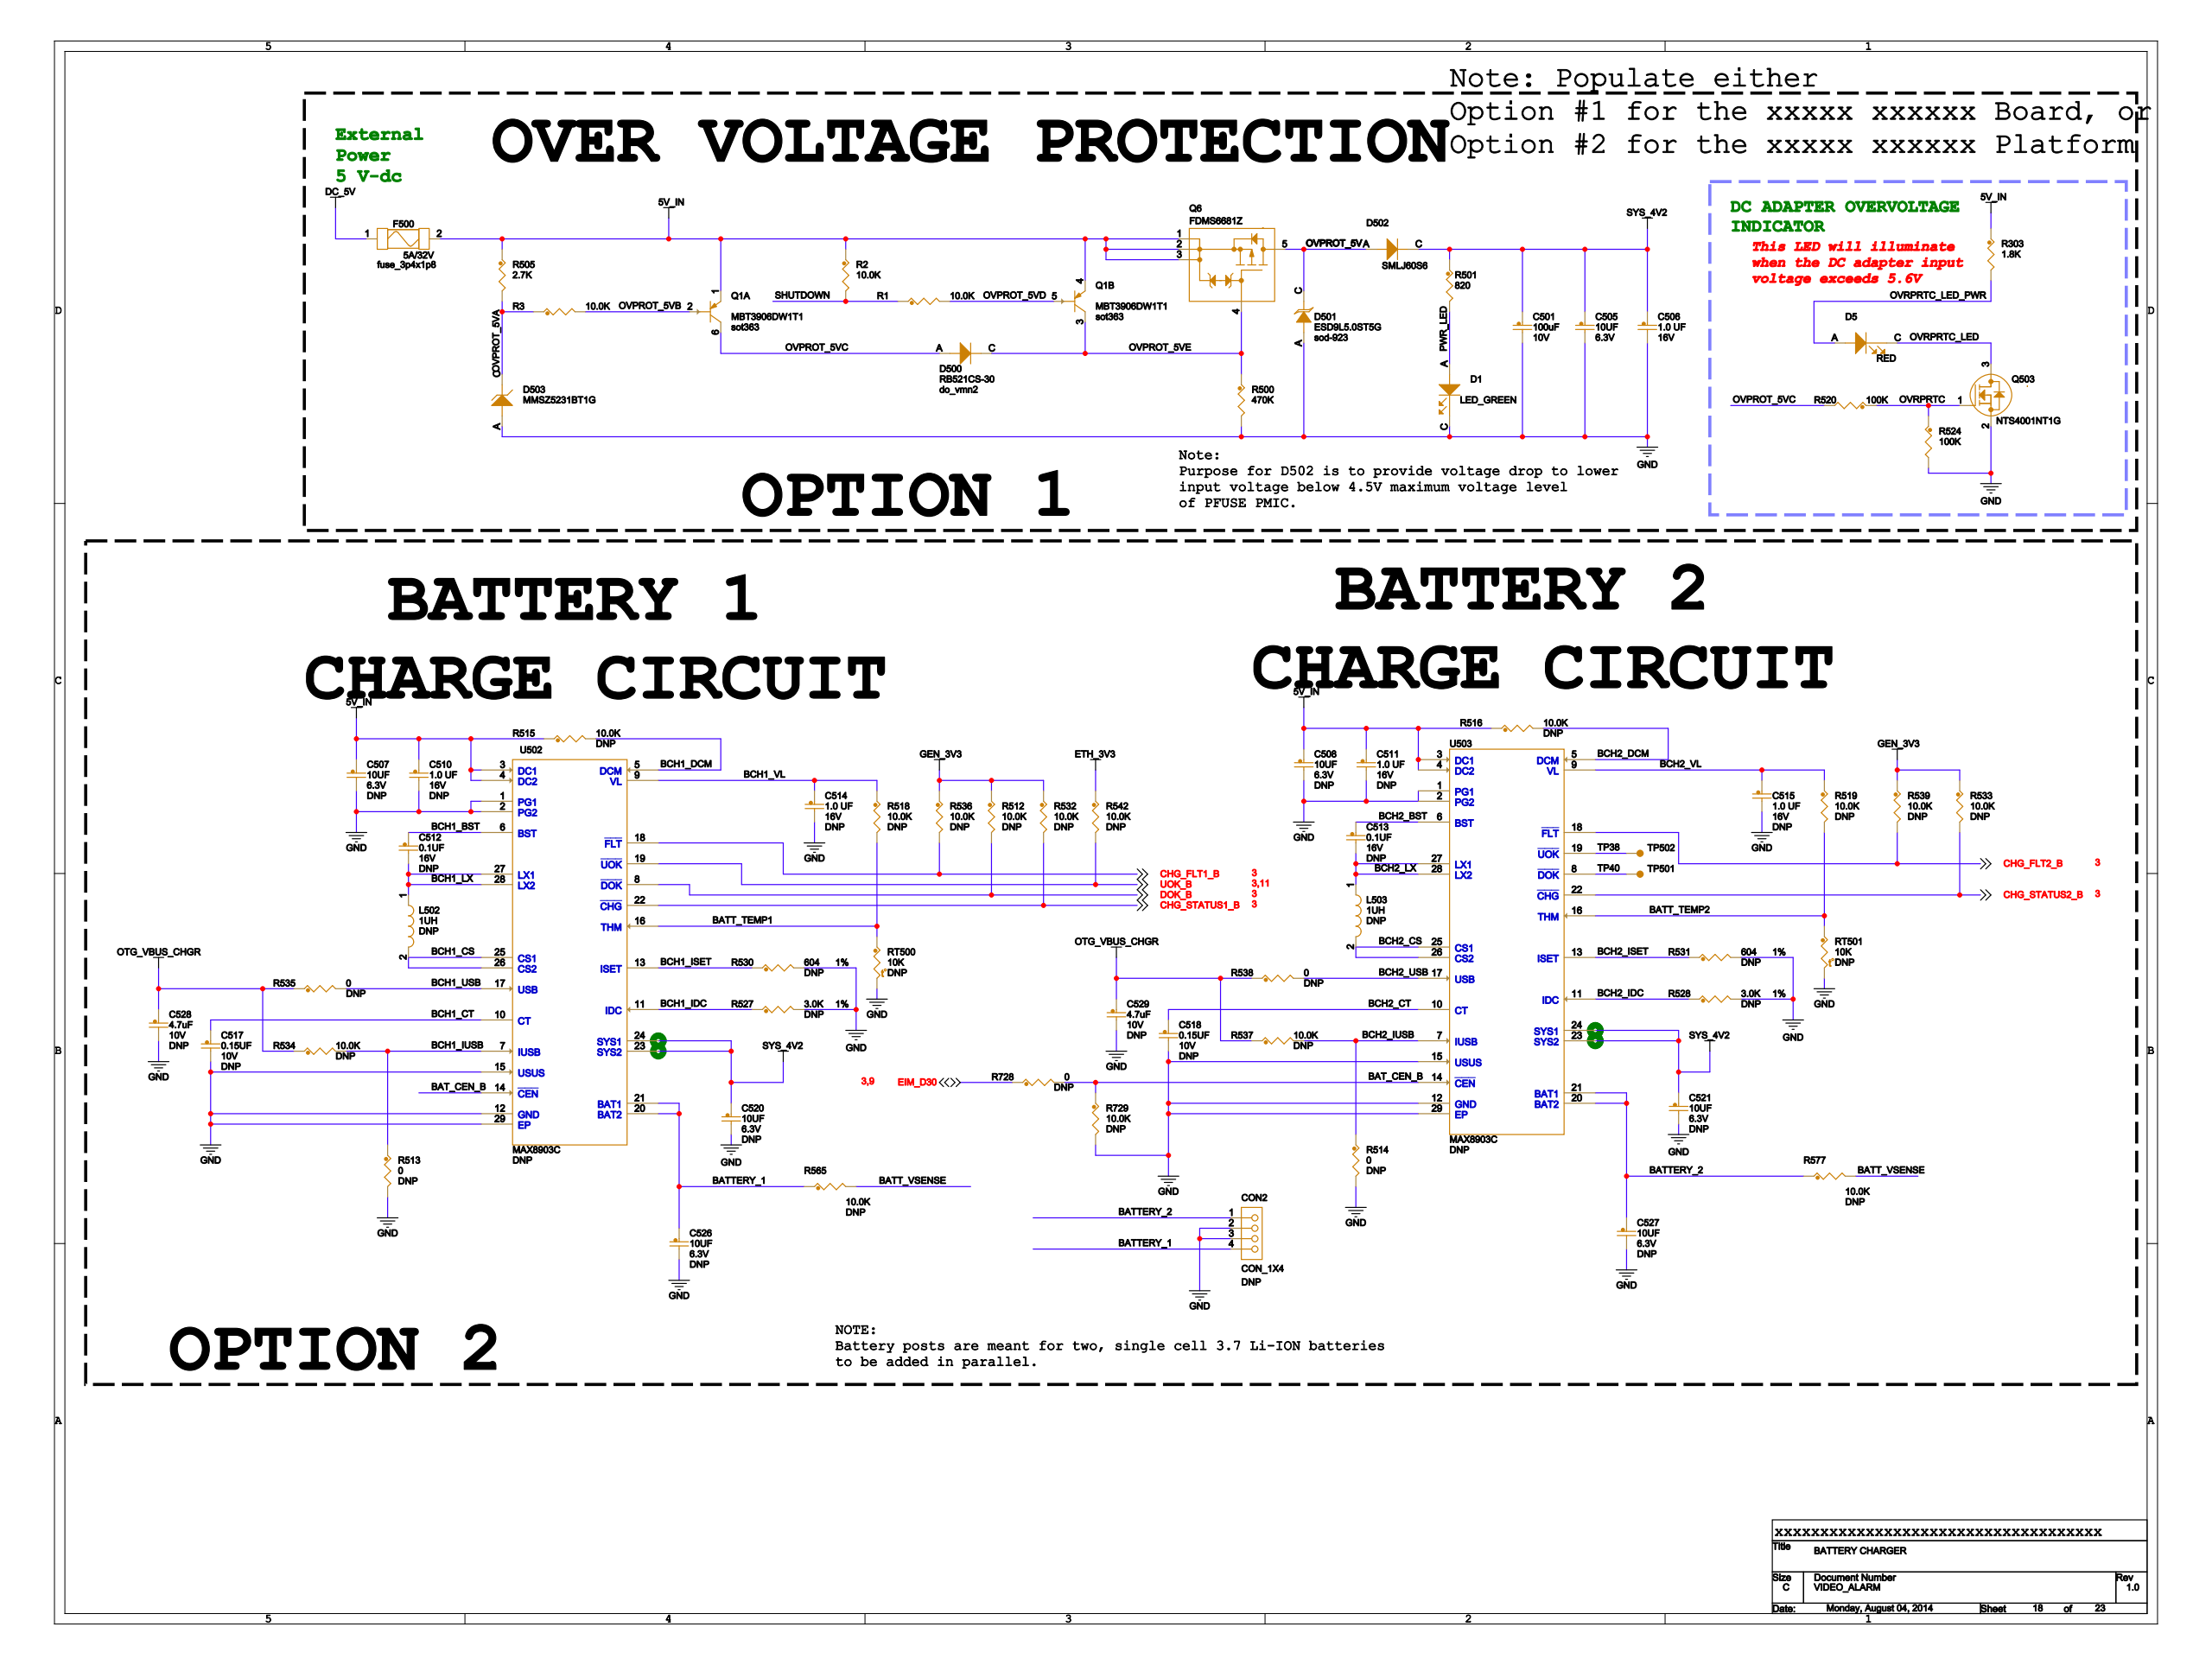Circuit board | Cadence Allegro | 994 parts | 728 nets | one sheet of the schematic
Parts on this sheet (reference | value | footprint):
C501 | 100uF | 1206_CC
C505 | 10UF | 0603_CC
C506 | 1.0 UF | 0603_CC
C507 | 10UF | 0603_CC
C508 | 10UF | 0603_CC
C510 | 1.0 UF | 0603_CC
C511 | 1.0 UF | 0603_CC
C512 | 0.1UF | 0603_CC
C513 | 0.1UF | 0603_CC
C514 | 1.0 UF | 0603_CC
C515 | 1.0 UF | 0603_CC
C517 | 0.15UF | 0603_CC
C518 | 0.15UF | 0603_CC
C520 | 10UF | 0603_CC
C521 | 10UF | 0603_CC
C526 | 10UF | 0603_CC
C527 | 10UF | 0603_CC
C528 | 4.7uF | 0603_CC
C529 | 4.7uF | 0603_CC
CON2 | CON_1X4 | BATTERY
D1 | LED_GREEN | LED_0603
D5 | RED | LED_0603
D500 | RB521CS-30 | DO_VMN2
D501 | ESD9L5.0ST5G | SOD-923
D502 | SMLJ60S6 | DO214AB_SM
D503 | MMSZ5231BT1G | SOD123
F500 | 5A/32V | FUSE_3P4X1P8
L502 | 1UH | IND_VLS252010
L503 | 1UH | IND_VLS252010
Q6 | FDMS6681Z | SO8_PAK
Q503 | NTS4001NT1G | SC70_3
R1 | 10.0K | 0603_CC
R2 | 10.0K | 0603_CC
R3 | 10.0K | 0603_CC
R303 | 1.8K | 0603_CC
R500 | 470K | 0603_CC
R501 | 820 | 0603_CC
R505 | 2.7K | 0603_CC
R512 | 10.0K | 0603_CC
R513 | 0 | 0603_CC
R514 | 0 | 0603_CC
R515 | 10.0K | 0603_CC
R516 | 10.0K | 0603_CC
R518 | 10.0K | 0603_CC
R519 | 10.0K | 0603_CC
R520 | 100K | 0603_CC
R524 | 100K | 0603_CC
R527 | 3.0K | 0603_CC
R528 | 3.0K | 0603_CC
R530 | 604 | 0603_CC
R531 | 604 | 0603_CC
R532 | 10.0K | 0603_CC
R533 | 10.0K | 0603_CC
R534 | 10.0K | 0603_CC
R535 | 0 | 0603_CC
R536 | 10.0K | 0603_CC
R537 | 10.0K | 0603_CC
R538 | 0 | 0603_CC
R539 | 10.0K | 0603_CC
R542 | 10.0K | 0603_CC
R565 | 10.0K | 0603_CC
R577 | 10.0K | 0603_CC
R728 | 0 | 0603_CC
R729 | 10.0K | 0603_CC
RT500 | 10K | 0603_CC
RT501 | 10K | 0603_CC
TP501 | TEST POINT | C035S
TP502 | TEST POINT | C035S
U502 | MAX8903C | TQFN28_0P4_4X4
U503 | MAX8903C | TQFN28_0P4_4X4
Nets of these parts (net: part-pin ...):
GND: C501-2 C505-2 C506-2 C507-2 C508-2 C510-2 C511-2 C514-2 C515-2 C517-2 C518-2 C520-2 C521-2 C526-2 C527-2 C528-2 C529-2 CON2-2 CON2-3 D1-C D501-A D503-A Q503-2 R500-2 R513-2 R514-2 R524-2 R527-2 R528-2 R530-2 R531-2 R729-2 RT500-2 RT501-2 U502-1 U502-2 U502-12 U502-15 U502-29 U503-1 U503-2 U503-12 U503-15 U503-29
GEN_3V3: R512-1 R532-1 R533-1 R536-1 R539-1
SYS_4V2: C501-1 C505-1 C506-1 C520-1 C521-1 D502-C R501-1 U502-23 U502-24 U503-23 U503-24
5V_IN: C507-1 C508-1 C510-1 C511-1 F500-2 Q6-1 Q6-2 Q6-3 R2-1 R303-1 R505-1 R515-1 R516-1 U502-3 U502-4 U503-3 U503-4
BATTERY_2: C527-1 CON2-1 R577-1 U503-20 U503-21
BATTERY_1: C526-1 CON2-4 R565-1 U502-20 U502-21
ETH_3V3: R542-1
PWR_LED: D1-A R501-2
OVRPRTC_LED_PWR: D5-A R303-2
OVRPRTC: Q503-1 R520-1 R524-1
OVPROT_5VC: D500-A R520-2
EIM_D30: R728-1
BAT_CEN_B: R728-2 R729-1 U502-14 U503-14
OTG_VBUS_CHGR: C528-1 C529-1 R534-1 R535-1 R537-1 R538-1
BCH2_USB: R538-2 U503-17
BCH1_USB: R535-2 U502-17
BCH2_IUSB: R514-1 R537-2 U503-7
BCH1_IUSB: R513-1 R534-2 U502-7
BATT_VSENSE: R565-2 R577-2
UOK_B: R542-2 U502-19
CHG_FLT2_B: R539-2 U503-18
CHG_FLT1_B: R536-2 U502-18
CHG_STATUS2_B: R533-2 U503-22
CHG_STATUS1_B: R532-2 U502-22
BCH2_VL: C515-1 R519-1 U503-9
BATT_TEMP2: R519-2 RT501-1 U503-16
BCH1_VL: C514-1 R518-1 U502-9
BATT_TEMP1: R518-2 RT500-1 U502-16
BCH2_DCM: R516-2 U503-5
BCH1_DCM: R515-2 U502-5
DOK_B: R512-2 U502-8
OVPROT_5VA: D503-C R3-1 R505-2
OVPROT_5VB: R3-2
SHUTDOWN: R1-1 R2-2
OVPROT_5VD: R1-2
DC_5V: F500-1
BCH2_BST: C513-1 U503-6
BCH2_LX: C513-2 L503-1 U503-27 U503-28
BCH1_BST: C512-1 U502-6
BCH1_LX: C512-2 L502-1 U502-27 U502-28
BCH2_CS: L503-2 U503-25 U503-26
BCH2_CT: C518-1 U503-10
TP40: TP501-1 U503-8
BCH2_IDC: R528-1 U503-11
BCH2_ISET: R531-1 U503-13
TP38: TP502-1 U503-19
BCH1_CS: L502-2 U502-25 U502-26
BCH1_CT: C517-1 U502-10
BCH1_IDC: R527-1 U502-11
BCH1_ISET: R530-1 U502-13
OVPROT_5VE: D500-C Q6-4 R500-1
OVPROT_5V: D501-C D502-A Q6-5
OVRPRTC_LED: D5-C Q503-3